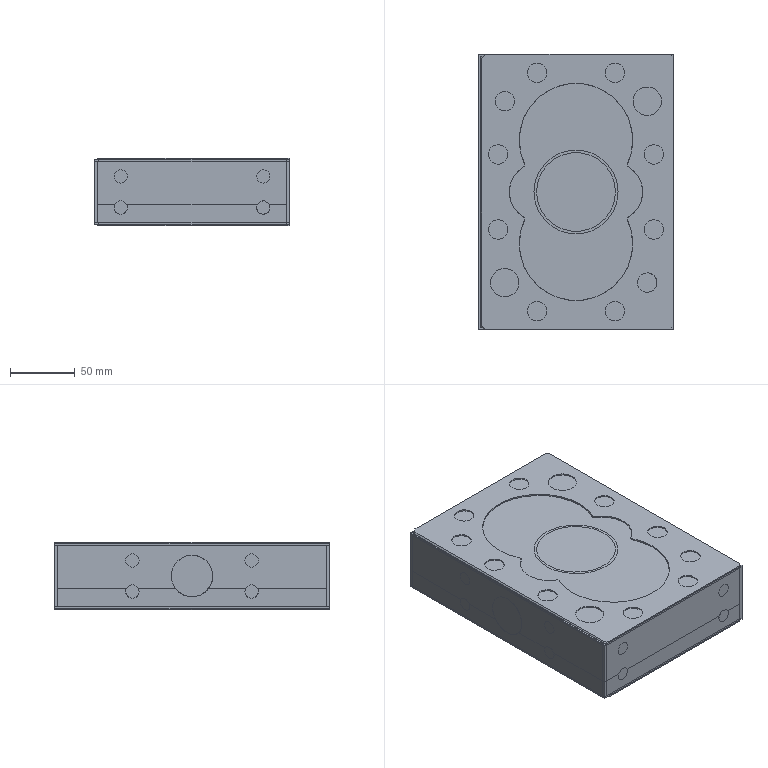NC program | NX | posted with a generic post | part box 150.2 x 212.2 x 52.4 mm
Whole program:
N10 G17 G21 G94 G90
(G81点孔_4 , TOOL : D6点孔钻_1)
N12 T01 M6
N14 /M1
N16 G54
N18 G17 G0 G90 X55. Y12. S1500 M3
N20 G43 Z20. H1
N22 G94 G81 G98 Z-1.5 F60. R1.5
N24 X-55.
N26 Y-12.
N28 X55.
N30 G80
N32 G0 X55. Y-12. Z20.
N34 M5
(G83钻孔_2 , TOOL : Z1.6钻头)
N36 T18 M6
N38 /M1
N40 G54
N42 G17 G0 G90 X55. Y12. S800 M3
N44 G43 Z20. H18
N46 G94 G83 G98 Z-35.165 F42. Q1. R1.5
N48 X-55. Z-30.918
N50 Y-12. Z-31.773
N52 X55. Z-35.165
N54 G80
N56 G0 X55. Y-12. Z20.
N58 M5
N60 M2